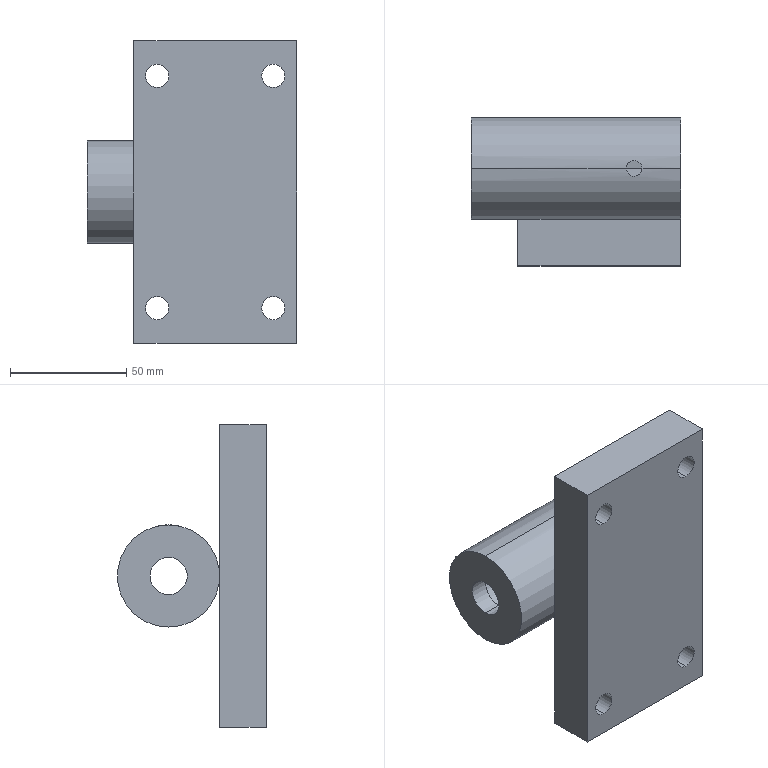Part | SolidWorks | features MirrorStock 1 | 2 solids | 25 faces | box 90 x 64 x 130 mm | volume 252738 mm3 | cylinder 16 | plane 9 | commonest cylinder face diameters 10 x8 6.8 x2 16 x2 30 x2 44 x2
STEP:
#1=CARTESIAN_POINT('',(-25.,20.,45.));
#2=VERTEX_POINT('',#1);
#3=CARTESIAN_POINT('',(-25.,20.,55.));
#4=VERTEX_POINT('',#3);
#5=CARTESIAN_POINT('',(-25.,20.,50.));
#6=DIRECTION('',(0.,-1.,0.));
#7=DIRECTION('',(0.,0.,-1.));
#8=AXIS2_PLACEMENT_3D('',#5,#6,#7);
#9=CIRCLE('',#8,5.);
#10=EDGE_CURVE('',#2,#4,#9,.T.);
#11=ORIENTED_EDGE('',*,*,#10,.F.);
#12=CARTESIAN_POINT('',(-25.,0.,45.));
#13=VERTEX_POINT('',#12);
#14=CARTESIAN_POINT('',(-25.,20.,45.));
#15=DIRECTION('',(0.,-1.,0.));
#16=VECTOR('',#15,1000.);
#17=LINE('',#14,#16);
#18=EDGE_CURVE('',#2,#13,#17,.T.);
#19=ORIENTED_EDGE('',*,*,#18,.T.);
#20=CARTESIAN_POINT('',(-25.,0.,55.));
#21=VERTEX_POINT('',#20);
#22=CARTESIAN_POINT('',(-25.,0.,50.));
#23=DIRECTION('',(0.,-1.,0.));
#24=DIRECTION('',(0.,0.,-1.));
#25=AXIS2_PLACEMENT_3D('',#22,#23,#24);
#26=CIRCLE('',#25,5.);
#27=EDGE_CURVE('',#13,#21,#26,.T.);
#28=ORIENTED_EDGE('',*,*,#27,.T.);
#29=CARTESIAN_POINT('',(-25.,20.,55.));
#30=DIRECTION('',(0.,-1.,0.));
#31=VECTOR('',#30,1000.);
#32=LINE('',#29,#31);
#33=EDGE_CURVE('',#4,#21,#32,.T.);
#34=ORIENTED_EDGE('',*,*,#33,.F.);
#35=EDGE_LOOP('',(#11,#19,#28,#34));
#36=FACE_OUTER_BOUND('',#35,.T.);
#37=CARTESIAN_POINT('',(-25.,20.,50.));
#38=DIRECTION('',(0.,-1.,0.));
#39=DIRECTION('',(0.,0.,1.));
#40=AXIS2_PLACEMENT_3D('',#37,#38,#39);
#41=CYLINDRICAL_SURFACE('',#40,5.);
#42=ADVANCED_FACE('',(#36),#41,.F.);
#43=CARTESIAN_POINT('',(25.,20.,45.));
#44=VERTEX_POINT('',#43);
#45=CARTESIAN_POINT('',(25.,20.,55.));
#46=VERTEX_POINT('',#45);
#47=CARTESIAN_POINT('',(25.,20.,50.));
#48=DIRECTION('',(0.,-1.,0.));
#49=DIRECTION('',(0.,0.,-1.));
#50=AXIS2_PLACEMENT_3D('',#47,#48,#49);
#51=CIRCLE('',#50,5.);
#52=EDGE_CURVE('',#44,#46,#51,.T.);
#53=ORIENTED_EDGE('',*,*,#52,.F.);
#54=CARTESIAN_POINT('',(25.,0.,45.));
#55=VERTEX_POINT('',#54);
#56=CARTESIAN_POINT('',(25.,20.,45.));
#57=DIRECTION('',(0.,-1.,0.));
#58=VECTOR('',#57,1000.);
#59=LINE('',#56,#58);
#60=EDGE_CURVE('',#44,#55,#59,.T.);
#61=ORIENTED_EDGE('',*,*,#60,.T.);
#62=CARTESIAN_POINT('',(25.,0.,55.));
#63=VERTEX_POINT('',#62);
#64=CARTESIAN_POINT('',(25.,0.,50.));
#65=DIRECTION('',(0.,-1.,0.));
#66=DIRECTION('',(0.,0.,-1.));
#67=AXIS2_PLACEMENT_3D('',#64,#65,#66);
#68=CIRCLE('',#67,5.);
#69=EDGE_CURVE('',#55,#63,#68,.T.);
#70=ORIENTED_EDGE('',*,*,#69,.T.);
#71=CARTESIAN_POINT('',(25.,20.,55.));
#72=DIRECTION('',(0.,-1.,0.));
#73=VECTOR('',#72,1000.);
#74=LINE('',#71,#73);
#75=EDGE_CURVE('',#46,#63,#74,.T.);
#76=ORIENTED_EDGE('',*,*,#75,.F.);
#77=EDGE_LOOP('',(#53,#61,#70,#76));
#78=FACE_OUTER_BOUND('',#77,.T.);
#79=CARTESIAN_POINT('',(25.,20.,50.));
#80=DIRECTION('',(0.,-1.,0.));
#81=DIRECTION('',(0.,0.,1.));
#82=AXIS2_PLACEMENT_3D('',#79,#80,#81);
#83=CYLINDRICAL_SURFACE('',#82,5.);
#84=ADVANCED_FACE('',(#78),#83,.F.);
#85=CARTESIAN_POINT('',(25.,20.,-55.));
#86=VERTEX_POINT('',#85);
#87=CARTESIAN_POINT('',(25.,20.,-45.));
#88=VERTEX_POINT('',#87);
#89=CARTESIAN_POINT('',(25.,20.,-50.));
#90=DIRECTION('',(0.,-1.,0.));
#91=DIRECTION('',(0.,0.,-1.));
#92=AXIS2_PLACEMENT_3D('',#89,#90,#91);
#93=CIRCLE('',#92,5.);
#94=EDGE_CURVE('',#86,#88,#93,.T.);
#95=ORIENTED_EDGE('',*,*,#94,.F.);
#96=CARTESIAN_POINT('',(25.,0.,-55.));
#97=VERTEX_POINT('',#96);
#98=CARTESIAN_POINT('',(25.,20.,-55.));
#99=DIRECTION('',(0.,-1.,0.));
#100=VECTOR('',#99,1000.);
#101=LINE('',#98,#100);
#102=EDGE_CURVE('',#86,#97,#101,.T.);
#103=ORIENTED_EDGE('',*,*,#102,.T.);
#104=CARTESIAN_POINT('',(25.,0.,-45.));
#105=VERTEX_POINT('',#104);
#106=CARTESIAN_POINT('',(25.,0.,-50.));
#107=DIRECTION('',(0.,-1.,0.));
#108=DIRECTION('',(0.,0.,-1.));
#109=AXIS2_PLACEMENT_3D('',#106,#107,#108);
#110=CIRCLE('',#109,5.);
#111=EDGE_CURVE('',#97,#105,#110,.T.);
#112=ORIENTED_EDGE('',*,*,#111,.T.);
#113=CARTESIAN_POINT('',(25.,20.,-45.));
#114=DIRECTION('',(0.,-1.,0.));
#115=VECTOR('',#114,1000.);
#116=LINE('',#113,#115);
#117=EDGE_CURVE('',#88,#105,#116,.T.);
#118=ORIENTED_EDGE('',*,*,#117,.F.);
#119=EDGE_LOOP('',(#95,#103,#112,#118));
#120=FACE_OUTER_BOUND('',#119,.T.);
#121=CARTESIAN_POINT('',(25.,20.,-50.));
#122=DIRECTION('',(0.,-1.,0.));
#123=DIRECTION('',(0.,0.,1.));
#124=AXIS2_PLACEMENT_3D('',#121,#122,#123);
#125=CYLINDRICAL_SURFACE('',#124,5.);
#126=ADVANCED_FACE('',(#120),#125,.F.);
#127=CARTESIAN_POINT('',(-25.,20.,-55.));
#128=VERTEX_POINT('',#127);
#129=CARTESIAN_POINT('',(-25.,20.,-45.));
#130=VERTEX_POINT('',#129);
#131=CARTESIAN_POINT('',(-25.,20.,-50.));
#132=DIRECTION('',(0.,-1.,0.));
#133=DIRECTION('',(0.,0.,-1.));
#134=AXIS2_PLACEMENT_3D('',#131,#132,#133);
#135=CIRCLE('',#134,5.);
#136=EDGE_CURVE('',#128,#130,#135,.T.);
#137=ORIENTED_EDGE('',*,*,#136,.F.);
#138=CARTESIAN_POINT('',(-25.,0.,-55.));
#139=VERTEX_POINT('',#138);
#140=CARTESIAN_POINT('',(-25.,20.,-55.));
#141=DIRECTION('',(0.,-1.,0.));
#142=VECTOR('',#141,1000.);
#143=LINE('',#140,#142);
#144=EDGE_CURVE('',#128,#139,#143,.T.);
#145=ORIENTED_EDGE('',*,*,#144,.T.);
#146=CARTESIAN_POINT('',(-25.,0.,-45.));
#147=VERTEX_POINT('',#146);
#148=CARTESIAN_POINT('',(-25.,0.,-50.));
#149=DIRECTION('',(0.,-1.,0.));
#150=DIRECTION('',(0.,0.,-1.));
#151=AXIS2_PLACEMENT_3D('',#148,#149,#150);
#152=CIRCLE('',#151,5.);
#153=EDGE_CURVE('',#139,#147,#152,.T.);
#154=ORIENTED_EDGE('',*,*,#153,.T.);
#155=CARTESIAN_POINT('',(-25.,20.,-45.));
#156=DIRECTION('',(0.,-1.,0.));
#157=VECTOR('',#156,1000.);
#158=LINE('',#155,#157);
#159=EDGE_CURVE('',#130,#147,#158,.T.);
#160=ORIENTED_EDGE('',*,*,#159,.F.);
#161=EDGE_LOOP('',(#137,#145,#154,#160));
#162=FACE_OUTER_BOUND('',#161,.T.);
#163=CARTESIAN_POINT('',(-25.,20.,-50.));
#164=DIRECTION('',(0.,-1.,0.));
#165=DIRECTION('',(0.,0.,1.));
#166=AXIS2_PLACEMENT_3D('',#163,#164,#165);
#167=CYLINDRICAL_SURFACE('',#166,5.);
#168=ADVANCED_FACE('',(#162),#167,.F.);
#169=CARTESIAN_POINT('',(-35.,20.,65.));
#170=VERTEX_POINT('',#169);
#171=CARTESIAN_POINT('',(-35.,20.,-65.));
#172=VERTEX_POINT('',#171);
#173=CARTESIAN_POINT('',(-35.,20.,-65.));
#174=DIRECTION('',(0.,0.,-1.));
#175=VECTOR('',#174,1000.);
#176=LINE('',#173,#175);
#177=EDGE_CURVE('',#170,#172,#176,.T.);
#178=ORIENTED_EDGE('',*,*,#177,.F.);
#179=CARTESIAN_POINT('',(35.,20.,65.));
#180=VERTEX_POINT('',#179);
#181=CARTESIAN_POINT('',(-35.,20.,65.));
#182=DIRECTION('',(-1.,0.,0.));
#183=VECTOR('',#182,1000.);
#184=LINE('',#181,#183);
#185=EDGE_CURVE('',#180,#170,#184,.T.);
#186=ORIENTED_EDGE('',*,*,#185,.F.);
#187=CARTESIAN_POINT('',(35.,20.,-65.));
#188=VERTEX_POINT('',#187);
#189=CARTESIAN_POINT('',(35.,20.,-65.));
#190=DIRECTION('',(0.,0.,1.));
#191=VECTOR('',#190,1000.);
#192=LINE('',#189,#191);
#193=EDGE_CURVE('',#188,#180,#192,.T.);
#194=ORIENTED_EDGE('',*,*,#193,.F.);
#195=CARTESIAN_POINT('',(-35.,20.,-65.));
#196=DIRECTION('',(1.,0.,0.));
#197=VECTOR('',#196,1000.);
#198=LINE('',#195,#197);
#199=EDGE_CURVE('',#172,#188,#198,.T.);
#200=ORIENTED_EDGE('',*,*,#199,.F.);
#201=EDGE_LOOP('',(#178,#186,#194,#200));
#202=FACE_OUTER_BOUND('',#201,.T.);
#203=CARTESIAN_POINT('',(25.,20.,50.));
#204=DIRECTION('',(0.,-1.,0.));
#205=DIRECTION('',(0.,0.,-1.));
#206=AXIS2_PLACEMENT_3D('',#203,#204,#205);
#207=CIRCLE('',#206,5.);
#208=EDGE_CURVE('',#46,#44,#207,.T.);
#209=ORIENTED_EDGE('',*,*,#208,.T.);
#210=ORIENTED_EDGE('',*,*,#52,.T.);
#211=EDGE_LOOP('',(#209,#210));
#212=FACE_BOUND('',#211,.T.);
#213=CARTESIAN_POINT('',(-25.,20.,50.));
#214=DIRECTION('',(0.,-1.,0.));
#215=DIRECTION('',(0.,0.,-1.));
#216=AXIS2_PLACEMENT_3D('',#213,#214,#215);
#217=CIRCLE('',#216,5.);
#218=EDGE_CURVE('',#4,#2,#217,.T.);
#219=ORIENTED_EDGE('',*,*,#218,.T.);
#220=ORIENTED_EDGE('',*,*,#10,.T.);
#221=EDGE_LOOP('',(#219,#220));
#222=FACE_BOUND('',#221,.T.);
#223=CARTESIAN_POINT('',(25.,20.,-50.));
#224=DIRECTION('',(0.,-1.,0.));
#225=DIRECTION('',(0.,0.,-1.));
#226=AXIS2_PLACEMENT_3D('',#223,#224,#225);
#227=CIRCLE('',#226,5.);
#228=EDGE_CURVE('',#88,#86,#227,.T.);
#229=ORIENTED_EDGE('',*,*,#228,.T.);
#230=ORIENTED_EDGE('',*,*,#94,.T.);
#231=EDGE_LOOP('',(#229,#230));
#232=FACE_BOUND('',#231,.T.);
#233=CARTESIAN_POINT('',(-25.,20.,-50.));
#234=DIRECTION('',(0.,-1.,0.));
#235=DIRECTION('',(0.,0.,-1.));
#236=AXIS2_PLACEMENT_3D('',#233,#234,#235);
#237=CIRCLE('',#236,5.);
#238=EDGE_CURVE('',#130,#128,#237,.T.);
#239=ORIENTED_EDGE('',*,*,#238,.T.);
#240=ORIENTED_EDGE('',*,*,#136,.T.);
#241=EDGE_LOOP('',(#239,#240));
#242=FACE_BOUND('',#241,.T.);
#243=CARTESIAN_POINT('',(0.,20.,0.));
#244=DIRECTION('',(0.,-1.,0.));
#245=DIRECTION('',(0.,0.,1.));
#246=AXIS2_PLACEMENT_3D('',#243,#244,#245);
#247=PLANE('',#246);
#248=ADVANCED_FACE('',(#202,#212,#222,#232,#242),#247,.F.);
#249=CARTESIAN_POINT('',(25.,0.,50.));
#250=DIRECTION('',(0.,-1.,0.));
#251=DIRECTION('',(0.,0.,-1.));
#252=AXIS2_PLACEMENT_3D('',#249,#250,#251);
#253=CIRCLE('',#252,5.);
#254=EDGE_CURVE('',#63,#55,#253,.T.);
#255=ORIENTED_EDGE('',*,*,#254,.F.);
#256=ORIENTED_EDGE('',*,*,#69,.F.);
#257=EDGE_LOOP('',(#255,#256));
#258=FACE_BOUND('',#257,.T.);
#259=CARTESIAN_POINT('',(-25.,0.,-50.));
#260=DIRECTION('',(0.,-1.,0.));
#261=DIRECTION('',(0.,0.,-1.));
#262=AXIS2_PLACEMENT_3D('',#259,#260,#261);
#263=CIRCLE('',#262,5.);
#264=EDGE_CURVE('',#147,#139,#263,.T.);
#265=ORIENTED_EDGE('',*,*,#264,.F.);
#266=ORIENTED_EDGE('',*,*,#153,.F.);
#267=EDGE_LOOP('',(#265,#266));
#268=FACE_BOUND('',#267,.T.);
#269=CARTESIAN_POINT('',(35.,0.,-65.));
#270=VERTEX_POINT('',#269);
#271=CARTESIAN_POINT('',(35.,0.,65.));
#272=VERTEX_POINT('',#271);
#273=CARTESIAN_POINT('',(35.,0.,-65.));
#274=DIRECTION('',(0.,0.,1.));
#275=VECTOR('',#274,1000.);
#276=LINE('',#273,#275);
#277=EDGE_CURVE('',#270,#272,#276,.T.);
#278=ORIENTED_EDGE('',*,*,#277,.T.);
#279=CARTESIAN_POINT('',(-35.,0.,65.));
#280=VERTEX_POINT('',#279);
#281=CARTESIAN_POINT('',(-35.,0.,65.));
#282=DIRECTION('',(-1.,0.,0.));
#283=VECTOR('',#282,1000.);
#284=LINE('',#281,#283);
#285=EDGE_CURVE('',#272,#280,#284,.T.);
#286=ORIENTED_EDGE('',*,*,#285,.T.);
#287=CARTESIAN_POINT('',(-35.,0.,-65.));
#288=VERTEX_POINT('',#287);
#289=CARTESIAN_POINT('',(-35.,0.,-65.));
#290=DIRECTION('',(0.,0.,-1.));
#291=VECTOR('',#290,1000.);
#292=LINE('',#289,#291);
#293=EDGE_CURVE('',#280,#288,#292,.T.);
#294=ORIENTED_EDGE('',*,*,#293,.T.);
#295=CARTESIAN_POINT('',(-35.,0.,-65.));
#296=DIRECTION('',(1.,0.,0.));
#297=VECTOR('',#296,1000.);
#298=LINE('',#295,#297);
#299=EDGE_CURVE('',#288,#270,#298,.T.);
#300=ORIENTED_EDGE('',*,*,#299,.T.);
#301=EDGE_LOOP('',(#278,#286,#294,#300));
#302=FACE_OUTER_BOUND('',#301,.T.);
#303=CARTESIAN_POINT('',(25.,0.,-50.));
#304=DIRECTION('',(0.,-1.,0.));
#305=DIRECTION('',(0.,0.,-1.));
#306=AXIS2_PLACEMENT_3D('',#303,#304,#305);
#307=CIRCLE('',#306,5.);
#308=EDGE_CURVE('',#105,#97,#307,.T.);
#309=ORIENTED_EDGE('',*,*,#308,.F.);
#310=ORIENTED_EDGE('',*,*,#111,.F.);
#311=EDGE_LOOP('',(#309,#310));
#312=FACE_BOUND('',#311,.T.);
#313=CARTESIAN_POINT('',(-25.,0.,50.));
#314=DIRECTION('',(0.,-1.,0.));
#315=DIRECTION('',(0.,0.,-1.));
#316=AXIS2_PLACEMENT_3D('',#313,#314,#315);
#317=CIRCLE('',#316,5.);
#318=EDGE_CURVE('',#21,#13,#317,.T.);
#319=ORIENTED_EDGE('',*,*,#318,.F.);
#320=ORIENTED_EDGE('',*,*,#27,.F.);
#321=EDGE_LOOP('',(#319,#320));
#322=FACE_BOUND('',#321,.T.);
#323=CARTESIAN_POINT('',(0.,0.,0.));
#324=DIRECTION('',(0.,-1.,0.));
#325=DIRECTION('',(0.,0.,1.));
#326=AXIS2_PLACEMENT_3D('',#323,#324,#325);
#327=PLANE('',#326);
#328=ADVANCED_FACE('',(#258,#268,#302,#312,#322),#327,.T.);
#329=ORIENTED_EDGE('',*,*,#277,.F.);
#330=CARTESIAN_POINT('',(35.,20.,-65.));
#331=DIRECTION('',(0.,-1.,0.));
#332=VECTOR('',#331,1000.);
#333=LINE('',#330,#332);
#334=EDGE_CURVE('',#188,#270,#333,.T.);
#335=ORIENTED_EDGE('',*,*,#334,.F.);
#336=ORIENTED_EDGE('',*,*,#193,.T.);
#337=CARTESIAN_POINT('',(35.,20.,65.));
#338=DIRECTION('',(0.,-1.,0.));
#339=VECTOR('',#338,1000.);
#340=LINE('',#337,#339);
#341=EDGE_CURVE('',#180,#272,#340,.T.);
#342=ORIENTED_EDGE('',*,*,#341,.T.);
#343=EDGE_LOOP('',(#329,#335,#336,#342));
#344=FACE_OUTER_BOUND('',#343,.T.);
#345=CARTESIAN_POINT('',(35.,20.,-65.));
#346=DIRECTION('',(-1.,0.,0.));
#347=DIRECTION('',(0.,0.,-1.));
#348=AXIS2_PLACEMENT_3D('',#345,#346,#347);
#349=PLANE('',#348);
#350=ADVANCED_FACE('',(#344),#349,.F.);
#351=ORIENTED_EDGE('',*,*,#285,.F.);
#352=ORIENTED_EDGE('',*,*,#341,.F.);
#353=ORIENTED_EDGE('',*,*,#185,.T.);
#354=CARTESIAN_POINT('',(-35.,20.,65.));
#355=DIRECTION('',(0.,-1.,0.));
#356=VECTOR('',#355,1000.);
#357=LINE('',#354,#356);
#358=EDGE_CURVE('',#170,#280,#357,.T.);
#359=ORIENTED_EDGE('',*,*,#358,.T.);
#360=EDGE_LOOP('',(#351,#352,#353,#359));
#361=FACE_OUTER_BOUND('',#360,.T.);
#362=CARTESIAN_POINT('',(-35.,20.,65.));
#363=DIRECTION('',(0.,0.,-1.));
#364=DIRECTION('',(1.,0.,0.));
#365=AXIS2_PLACEMENT_3D('',#362,#363,#364);
#366=PLANE('',#365);
#367=ADVANCED_FACE('',(#361),#366,.F.);
#368=ORIENTED_EDGE('',*,*,#293,.F.);
#369=ORIENTED_EDGE('',*,*,#358,.F.);
#370=ORIENTED_EDGE('',*,*,#177,.T.);
#371=CARTESIAN_POINT('',(-35.,20.,-65.));
#372=DIRECTION('',(0.,-1.,0.));
#373=VECTOR('',#372,1000.);
#374=LINE('',#371,#373);
#375=EDGE_CURVE('',#172,#288,#374,.T.);
#376=ORIENTED_EDGE('',*,*,#375,.T.);
#377=EDGE_LOOP('',(#368,#369,#370,#376));
#378=FACE_OUTER_BOUND('',#377,.T.);
#379=CARTESIAN_POINT('',(-35.,20.,-65.));
#380=DIRECTION('',(1.,0.,0.));
#381=DIRECTION('',(0.,0.,1.));
#382=AXIS2_PLACEMENT_3D('',#379,#380,#381);
#383=PLANE('',#382);
#384=ADVANCED_FACE('',(#378),#383,.F.);
#385=ORIENTED_EDGE('',*,*,#299,.F.);
#386=ORIENTED_EDGE('',*,*,#375,.F.);
#387=ORIENTED_EDGE('',*,*,#199,.T.);
#388=ORIENTED_EDGE('',*,*,#334,.T.);
#389=EDGE_LOOP('',(#385,#386,#387,#388));
#390=FACE_OUTER_BOUND('',#389,.T.);
#391=CARTESIAN_POINT('',(-35.,20.,-65.));
#392=DIRECTION('',(0.,0.,1.));
#393=DIRECTION('',(-1.,0.,0.));
#394=AXIS2_PLACEMENT_3D('',#391,#392,#393);
#395=PLANE('',#394);
#396=ADVANCED_FACE('',(#390),#395,.F.);
#397=ORIENTED_EDGE('',*,*,#144,.F.);
#398=ORIENTED_EDGE('',*,*,#238,.F.);
#399=ORIENTED_EDGE('',*,*,#159,.T.);
#400=ORIENTED_EDGE('',*,*,#264,.T.);
#401=EDGE_LOOP('',(#397,#398,#399,#400));
#402=FACE_OUTER_BOUND('',#401,.T.);
#403=CARTESIAN_POINT('',(-25.,20.,-50.));
#404=DIRECTION('',(0.,-1.,0.));
#405=DIRECTION('',(0.,0.,1.));
#406=AXIS2_PLACEMENT_3D('',#403,#404,#405);
#407=CYLINDRICAL_SURFACE('',#406,5.);
#408=ADVANCED_FACE('',(#402),#407,.F.);
#409=ORIENTED_EDGE('',*,*,#102,.F.);
#410=ORIENTED_EDGE('',*,*,#228,.F.);
#411=ORIENTED_EDGE('',*,*,#117,.T.);
#412=ORIENTED_EDGE('',*,*,#308,.T.);
#413=EDGE_LOOP('',(#409,#410,#411,#412));
#414=FACE_OUTER_BOUND('',#413,.T.);
#415=CARTESIAN_POINT('',(25.,20.,-50.));
#416=DIRECTION('',(0.,-1.,0.));
#417=DIRECTION('',(0.,0.,1.));
#418=AXIS2_PLACEMENT_3D('',#415,#416,#417);
#419=CYLINDRICAL_SURFACE('',#418,5.);
#420=ADVANCED_FACE('',(#414),#419,.F.);
#421=ORIENTED_EDGE('',*,*,#60,.F.);
#422=ORIENTED_EDGE('',*,*,#208,.F.);
#423=ORIENTED_EDGE('',*,*,#75,.T.);
#424=ORIENTED_EDGE('',*,*,#254,.T.);
#425=EDGE_LOOP('',(#421,#422,#423,#424));
#426=FACE_OUTER_BOUND('',#425,.T.);
#427=CARTESIAN_POINT('',(25.,20.,50.));
#428=DIRECTION('',(0.,-1.,0.));
#429=DIRECTION('',(0.,0.,1.));
#430=AXIS2_PLACEMENT_3D('',#427,#428,#429);
#431=CYLINDRICAL_SURFACE('',#430,5.);
#432=ADVANCED_FACE('',(#426),#431,.F.);
#433=ORIENTED_EDGE('',*,*,#18,.F.);
#434=ORIENTED_EDGE('',*,*,#218,.F.);
#435=ORIENTED_EDGE('',*,*,#33,.T.);
#436=ORIENTED_EDGE('',*,*,#318,.T.);
#437=EDGE_LOOP('',(#433,#434,#435,#436));
#438=FACE_OUTER_BOUND('',#437,.T.);
#439=CARTESIAN_POINT('',(-25.,20.,50.));
#440=DIRECTION('',(0.,-1.,0.));
#441=DIRECTION('',(0.,0.,1.));
#442=AXIS2_PLACEMENT_3D('',#439,#440,#441);
#443=CYLINDRICAL_SURFACE('',#442,5.);
#444=ADVANCED_FACE('',(#438),#443,.F.);
#445=CLOSED_SHELL('',(#42,#84,#126,#168,#248,#328,#350,#367,#384,#396,#408,#420,#432,#444));
#446=MANIFOLD_SOLID_BREP('',#445);
#447=CARTESIAN_POINT('',(18.4,42.,22.));
#448=VERTEX_POINT('',#447);
#449=CARTESIAN_POINT('',(11.6,42.,22.));
#450=VERTEX_POINT('',#449);
#451=CARTESIAN_POINT('',(18.4,42.,22.));
#452=CARTESIAN_POINT('',(18.4,42.225,22.));
#453=CARTESIAN_POINT('',(18.378,42.446,21.997));
#454=CARTESIAN_POINT('',(18.291,42.881,21.983));
#455=CARTESIAN_POINT('',(18.226,43.097,21.974));
#456=CARTESIAN_POINT('',(18.055,43.509,21.949));
#457=CARTESIAN_POINT('',(17.95,43.704,21.935));
#458=CARTESIAN_POINT('',(17.704,44.074,21.903));
#459=CARTESIAN_POINT('',(17.56,44.248,21.885));
#460=CARTESIAN_POINT('',(17.247,44.561,21.851));
#461=CARTESIAN_POINT('',(17.076,44.702,21.834));
#462=CARTESIAN_POINT('',(16.704,44.95,21.802));
#463=CARTESIAN_POINT('',(16.507,45.056,21.787));
#464=CARTESIAN_POINT('',(16.098,45.225,21.762));
#465=CARTESIAN_POINT('',(15.883,45.291,21.753));
#466=CARTESIAN_POINT('',(15.444,45.378,21.739));
#467=CARTESIAN_POINT('',(15.223,45.4,21.736));
#468=CARTESIAN_POINT('',(14.779,45.4,21.736));
#469=CARTESIAN_POINT('',(14.553,45.378,21.739));
#470=CARTESIAN_POINT('',(14.117,45.291,21.753));
#471=CARTESIAN_POINT('',(13.905,45.227,21.762));
#472=CARTESIAN_POINT('',(13.493,45.056,21.787));
#473=CARTESIAN_POINT('',(13.294,44.95,21.802));
#474=CARTESIAN_POINT('',(12.926,44.704,21.834));
#475=CARTESIAN_POINT('',(12.754,44.563,21.851));
#476=CARTESIAN_POINT('',(12.438,44.246,21.886));
#477=CARTESIAN_POINT('',(12.297,44.074,21.903));
#478=CARTESIAN_POINT('',(12.051,43.707,21.934));
#479=CARTESIAN_POINT('',(11.944,43.508,21.949));
#480=CARTESIAN_POINT('',(11.774,43.096,21.974));
#481=CARTESIAN_POINT('',(11.709,42.884,21.983));
#482=CARTESIAN_POINT('',(11.622,42.448,21.997));
#483=CARTESIAN_POINT('',(11.6,42.222,22.));
#484=CARTESIAN_POINT('',(11.6,42.,22.));
#485=B_SPLINE_CURVE_WITH_KNOTS('',3,(#451,#452,#453,#454,#455,#456,#457,#458,#459,#460,#461,#462,#463,#464,#465,#466,#467,#468,#469,#470,#471,#472,#473,#474,#475,#476,#477,#478,#479,#480,#481,#482,#483,#484),.UNSPECIFIED.,.F.,.F.,(4,2,2,2,2,2,2,2,2,2,2,2,2,2,2,2,4),(0.,0.0006654,0.001331,0.001996,0.002661,0.003327,0.003992,0.004658,0.005323,0.005988,0.006654,0.007319,0.007984,0.00865,0.009315,0.009981,0.01065),.UNSPECIFIED.);
#486=EDGE_CURVE('',#448,#450,#485,.T.);
#487=ORIENTED_EDGE('',*,*,#486,.T.);
#488=CARTESIAN_POINT('',(11.6,42.,15.));
#489=VERTEX_POINT('',#488);
#490=CARTESIAN_POINT('',(11.6,42.,0.));
#491=DIRECTION('',(0.,0.,-1.));
#492=VECTOR('',#491,1000.);
#493=LINE('',#490,#492);
#494=EDGE_CURVE('',#450,#489,#493,.T.);
#495=ORIENTED_EDGE('',*,*,#494,.T.);
#496=CARTESIAN_POINT('',(18.4,42.,15.));
#497=VERTEX_POINT('',#496);
#498=CARTESIAN_POINT('',(11.6,42.,15.));
#499=CARTESIAN_POINT('',(11.6,42.222,15.));
#500=CARTESIAN_POINT('',(11.622,42.444,14.995));
#501=CARTESIAN_POINT('',(11.709,42.885,14.976));
#502=CARTESIAN_POINT('',(11.775,43.098,14.961));
#503=CARTESIAN_POINT('',(11.944,43.507,14.925));
#504=CARTESIAN_POINT('',(12.051,43.706,14.904));
#505=CARTESIAN_POINT('',(12.298,44.076,14.857));
#506=CARTESIAN_POINT('',(12.438,44.246,14.832));
#507=CARTESIAN_POINT('',(12.751,44.56,14.781));
#508=CARTESIAN_POINT('',(12.926,44.703,14.755));
#509=CARTESIAN_POINT('',(13.293,44.949,14.708));
#510=CARTESIAN_POINT('',(13.488,45.054,14.686));
#511=CARTESIAN_POINT('',(14.108,45.311,14.631));
#512=CARTESIAN_POINT('',(14.55,45.4,14.61));
#513=CARTESIAN_POINT('',(15.223,45.4,14.61));
#514=CARTESIAN_POINT('',(15.444,45.378,14.615));
#515=CARTESIAN_POINT('',(15.88,45.292,14.634));
#516=CARTESIAN_POINT('',(16.097,45.226,14.649));
#517=CARTESIAN_POINT('',(16.508,45.056,14.686));
#518=CARTESIAN_POINT('',(16.703,44.951,14.707));
#519=CARTESIAN_POINT('',(17.073,44.704,14.755));
#520=CARTESIAN_POINT('',(17.246,44.562,14.78));
#521=CARTESIAN_POINT('',(17.559,44.25,14.831));
#522=CARTESIAN_POINT('',(17.7,44.078,14.857));
#523=CARTESIAN_POINT('',(17.949,43.706,14.904));
#524=CARTESIAN_POINT('',(18.054,43.511,14.925));
#525=CARTESIAN_POINT('',(18.224,43.102,14.961));
#526=CARTESIAN_POINT('',(18.29,42.886,14.975));
#527=CARTESIAN_POINT('',(18.378,42.448,14.995));
#528=CARTESIAN_POINT('',(18.4,42.225,15.));
#529=CARTESIAN_POINT('',(18.4,42.,15.));
#530=B_SPLINE_CURVE_WITH_KNOTS('',3,(#498,#499,#500,#501,#502,#503,#504,#505,#506,#507,#508,#509,#510,#511,#512,#513,#514,#515,#516,#517,#518,#519,#520,#521,#522,#523,#524,#525,#526,#527,#528,#529),.UNSPECIFIED.,.F.,.F.,(4,2,2,2,2,2,2,2,2,2,2,2,2,2,2,4),(0.01066,0.01133,0.012,0.01266,0.01333,0.014,0.01466,0.016,0.01666,0.01733,0.01799,0.01866,0.01933,0.01999,0.02066,0.02133),.UNSPECIFIED.);
#531=EDGE_CURVE('',#489,#497,#530,.T.);
#532=ORIENTED_EDGE('',*,*,#531,.T.);
#533=CARTESIAN_POINT('',(18.4,42.,0.));
#534=DIRECTION('',(0.,0.,-1.));
#535=VECTOR('',#534,1000.);
#536=LINE('',#533,#535);
#537=EDGE_CURVE('',#448,#497,#536,.T.);
#538=ORIENTED_EDGE('',*,*,#537,.F.);
#539=EDGE_LOOP('',(#487,#495,#532,#538));
#540=FACE_OUTER_BOUND('',#539,.T.);
#541=CARTESIAN_POINT('',(15.,42.,0.));
#542=DIRECTION('',(0.,0.,-1.));
#543=DIRECTION('',(1.,0.,0.));
#544=AXIS2_PLACEMENT_3D('',#541,#542,#543);
#545=CYLINDRICAL_SURFACE('',#544,3.4);
#546=ADVANCED_FACE('',(#540),#545,.F.);
#547=CARTESIAN_POINT('',(-47.,42.,-8.));
#548=VERTEX_POINT('',#547);
#549=CARTESIAN_POINT('',(-47.,42.,8.));
#550=VERTEX_POINT('',#549);
#551=CARTESIAN_POINT('',(-47.,42.,0.));
#552=DIRECTION('',(1.,0.,0.));
#553=DIRECTION('',(0.,0.,-1.));
#554=AXIS2_PLACEMENT_3D('',#551,#552,#553);
#555=CIRCLE('',#554,8.);
#556=EDGE_CURVE('',#548,#550,#555,.T.);
#557=ORIENTED_EDGE('',*,*,#556,.T.);
#558=CARTESIAN_POINT('',(-55.,42.,8.));
#559=VERTEX_POINT('',#558);
#560=CARTESIAN_POINT('',(-55.,42.,8.));
#561=DIRECTION('',(-1.,0.,0.));
#562=VECTOR('',#561,1000.);
#563=LINE('',#560,#562);
#564=EDGE_CURVE('',#550,#559,#563,.T.);
#565=ORIENTED_EDGE('',*,*,#564,.T.);
#566=CARTESIAN_POINT('',(-55.,42.,-8.));
#567=VERTEX_POINT('',#566);
#568=CARTESIAN_POINT('',(-55.,42.,0.));
#569=DIRECTION('',(1.,0.,0.));
#570=DIRECTION('',(0.,0.,-1.));
#571=AXIS2_PLACEMENT_3D('',#568,#569,#570);
#572=CIRCLE('',#571,8.);
#573=EDGE_CURVE('',#567,#559,#572,.T.);
#574=ORIENTED_EDGE('',*,*,#573,.F.);
#575=CARTESIAN_POINT('',(-55.,42.,-8.));
#576=DIRECTION('',(-1.,0.,0.));
#577=VECTOR('',#576,1000.);
#578=LINE('',#575,#577);
#579=EDGE_CURVE('',#548,#567,#578,.T.);
#580=ORIENTED_EDGE('',*,*,#579,.F.);
#581=EDGE_LOOP('',(#557,#565,#574,#580));
#582=FACE_OUTER_BOUND('',#581,.T.);
#583=CARTESIAN_POINT('',(-55.,42.,0.));
#584=DIRECTION('',(-1.,0.,0.));
#585=DIRECTION('',(0.,0.,-1.));
#586=AXIS2_PLACEMENT_3D('',#583,#584,#585);
#587=CYLINDRICAL_SURFACE('',#586,8.);
#588=ADVANCED_FACE('',(#582),#587,.F.);
#589=CARTESIAN_POINT('',(35.,42.,22.));
#590=VERTEX_POINT('',#589);
#591=CARTESIAN_POINT('',(35.,42.,-22.));
#592=VERTEX_POINT('',#591);
#593=CARTESIAN_POINT('',(35.,42.,0.));
#594=DIRECTION('',(1.,0.,0.));
#595=DIRECTION('',(0.,0.,-1.));
#596=AXIS2_PLACEMENT_3D('',#593,#594,#595);
#597=CIRCLE('',#596,22.);
#598=EDGE_CURVE('',#590,#592,#597,.T.);
#599=ORIENTED_EDGE('',*,*,#598,.F.);
#600=CARTESIAN_POINT('',(-55.,42.,22.));
#601=DIRECTION('',(-1.,0.,0.));
#602=VECTOR('',#601,1000.);
#603=LINE('',#600,#602);
#604=EDGE_CURVE('',#590,#448,#603,.T.);
#605=ORIENTED_EDGE('',*,*,#604,.T.);
#606=CARTESIAN_POINT('',(11.6,42.,22.));
#607=CARTESIAN_POINT('',(11.6,41.778,22.));
#608=CARTESIAN_POINT('',(11.622,41.557,21.997));
#609=CARTESIAN_POINT('',(11.709,41.118,21.983));
#610=CARTESIAN_POINT('',(11.774,40.903,21.974));
#611=CARTESIAN_POINT('',(11.944,40.494,21.949));
#612=CARTESIAN_POINT('',(12.049,40.296,21.935));
#613=CARTESIAN_POINT('',(12.297,39.925,21.903));
#614=CARTESIAN_POINT('',(12.438,39.754,21.886));
#615=CARTESIAN_POINT('',(12.751,39.441,21.851));
#616=CARTESIAN_POINT('',(12.926,39.297,21.834));
#617=CARTESIAN_POINT('',(13.294,39.051,21.802));
#618=CARTESIAN_POINT('',(13.489,38.946,21.787));
#619=CARTESIAN_POINT('',(13.901,38.775,21.762));
#620=CARTESIAN_POINT('',(14.117,38.709,21.753));
#621=CARTESIAN_POINT('',(14.551,38.622,21.739));
#622=CARTESIAN_POINT('',(14.773,38.6,21.736));
#623=CARTESIAN_POINT('',(15.223,38.6,21.736));
#624=CARTESIAN_POINT('',(15.444,38.622,21.739));
#625=CARTESIAN_POINT('',(15.879,38.708,21.752));
#626=CARTESIAN_POINT('',(16.095,38.773,21.762));
#627=CARTESIAN_POINT('',(16.506,38.944,21.787));
#628=CARTESIAN_POINT('',(16.702,39.048,21.801));
#629=CARTESIAN_POINT('',(17.071,39.295,21.833));
#630=CARTESIAN_POINT('',(17.246,39.438,21.851));
#631=CARTESIAN_POINT('',(17.559,39.751,21.885));
#632=CARTESIAN_POINT('',(17.7,39.921,21.902));
#633=CARTESIAN_POINT('',(17.949,40.293,21.934));
#634=CARTESIAN_POINT('',(18.054,40.49,21.949));
#635=CARTESIAN_POINT('',(18.224,40.899,21.973));
#636=CARTESIAN_POINT('',(18.29,41.114,21.983));
#637=CARTESIAN_POINT('',(18.378,41.553,21.997));
#638=CARTESIAN_POINT('',(18.4,41.775,22.));
#639=CARTESIAN_POINT('',(18.4,42.,22.));
#640=B_SPLINE_CURVE_WITH_KNOTS('',3,(#606,#607,#608,#609,#610,#611,#612,#613,#614,#615,#616,#617,#618,#619,#620,#621,#622,#623,#624,#625,#626,#627,#628,#629,#630,#631,#632,#633,#634,#635,#636,#637,#638,#639),.UNSPECIFIED.,.F.,.F.,(4,2,2,2,2,2,2,2,2,2,2,2,2,2,2,2,4),(0.01065,0.01131,0.01198,0.01264,0.01331,0.01397,0.01464,0.0153,0.01597,0.01663,0.0173,0.01796,0.01863,0.01929,0.01996,0.02062,0.02129),.UNSPECIFIED.);
#641=EDGE_CURVE('',#450,#448,#640,.T.);
#642=ORIENTED_EDGE('',*,*,#641,.F.);
#643=CARTESIAN_POINT('',(-55.,42.,22.));
#644=VERTEX_POINT('',#643);
#645=CARTESIAN_POINT('',(-55.,42.,22.));
#646=DIRECTION('',(-1.,0.,0.));
#647=VECTOR('',#646,1000.);
#648=LINE('',#645,#647);
#649=EDGE_CURVE('',#450,#644,#648,.T.);
#650=ORIENTED_EDGE('',*,*,#649,.T.);
#651=CARTESIAN_POINT('',(-55.,42.,-22.));
#652=VERTEX_POINT('',#651);
#653=CARTESIAN_POINT('',(-55.,42.,0.));
#654=DIRECTION('',(1.,0.,0.));
#655=DIRECTION('',(0.,0.,-1.));
#656=AXIS2_PLACEMENT_3D('',#653,#654,#655);
#657=CIRCLE('',#656,22.);
#658=EDGE_CURVE('',#644,#652,#657,.T.);
#659=ORIENTED_EDGE('',*,*,#658,.T.);
#660=CARTESIAN_POINT('',(-55.,42.,-22.));
#661=DIRECTION('',(-1.,0.,0.));
#662=VECTOR('',#661,1000.);
#663=LINE('',#660,#662);
#664=EDGE_CURVE('',#592,#652,#663,.T.);
#665=ORIENTED_EDGE('',*,*,#664,.F.);
#666=EDGE_LOOP('',(#599,#605,#642,#650,#659,#665));
#667=FACE_OUTER_BOUND('',#666,.T.);
#668=CARTESIAN_POINT('',(-55.,42.,0.));
#669=DIRECTION('',(-1.,0.,0.));
#670=DIRECTION('',(0.,0.,-1.));
#671=AXIS2_PLACEMENT_3D('',#668,#669,#670);
#672=CYLINDRICAL_SURFACE('',#671,22.);
#673=ADVANCED_FACE('',(#667),#672,.T.);
#674=CARTESIAN_POINT('',(35.,42.,-15.));
#675=VERTEX_POINT('',#674);
#676=CARTESIAN_POINT('',(35.,42.,15.));
#677=VERTEX_POINT('',#676);
#678=CARTESIAN_POINT('',(35.,42.,0.));
#679=DIRECTION('',(1.,0.,0.));
#680=DIRECTION('',(0.,0.,-1.));
#681=AXIS2_PLACEMENT_3D('',#678,#679,#680);
#682=CIRCLE('',#681,15.);
#683=EDGE_CURVE('',#675,#677,#682,.T.);
#684=ORIENTED_EDGE('',*,*,#683,.T.);
#685=CARTESIAN_POINT('',(-55.,42.,15.));
#686=DIRECTION('',(-1.,0.,0.));
#687=VECTOR('',#686,1000.);
#688=LINE('',#685,#687);
#689=EDGE_CURVE('',#677,#497,#688,.T.);
#690=ORIENTED_EDGE('',*,*,#689,.T.);
#691=ORIENTED_EDGE('',*,*,#531,.F.);
#692=CARTESIAN_POINT('',(-47.,42.,15.));
#693=VERTEX_POINT('',#692);
#694=CARTESIAN_POINT('',(-55.,42.,15.));
#695=DIRECTION('',(-1.,0.,0.));
#696=VECTOR('',#695,1000.);
#697=LINE('',#694,#696);
#698=EDGE_CURVE('',#489,#693,#697,.T.);
#699=ORIENTED_EDGE('',*,*,#698,.T.);
#700=CARTESIAN_POINT('',(-47.,42.,-15.));
#701=VERTEX_POINT('',#700);
#702=CARTESIAN_POINT('',(-47.,42.,0.));
#703=DIRECTION('',(1.,0.,0.));
#704=DIRECTION('',(0.,0.,-1.));
#705=AXIS2_PLACEMENT_3D('',#702,#703,#704);
#706=CIRCLE('',#705,15.);
#707=EDGE_CURVE('',#701,#693,#706,.T.);
#708=ORIENTED_EDGE('',*,*,#707,.F.);
#709=CARTESIAN_POINT('',(-55.,42.,-15.));
#710=DIRECTION('',(-1.,0.,0.));
#711=VECTOR('',#710,1000.);
#712=LINE('',#709,#711);
#713=EDGE_CURVE('',#675,#701,#712,.T.);
#714=ORIENTED_EDGE('',*,*,#713,.F.);
#715=EDGE_LOOP('',(#684,#690,#691,#699,#708,#714));
#716=FACE_OUTER_BOUND('',#715,.T.);
#717=CARTESIAN_POINT('',(-55.,42.,0.));
#718=DIRECTION('',(-1.,0.,0.));
#719=DIRECTION('',(0.,0.,-1.));
#720=AXIS2_PLACEMENT_3D('',#717,#718,#719);
#721=CYLINDRICAL_SURFACE('',#720,15.);
#722=ADVANCED_FACE('',(#716),#721,.F.);
#723=ORIENTED_EDGE('',*,*,#707,.T.);
#724=CARTESIAN_POINT('',(-47.,42.,0.));
#725=DIRECTION('',(1.,0.,0.));
#726=DIRECTION('',(0.,0.,-1.));
#727=AXIS2_PLACEMENT_3D('',#724,#725,#726);
#728=CIRCLE('',#727,15.);
#729=EDGE_CURVE('',#693,#701,#728,.T.);
#730=ORIENTED_EDGE('',*,*,#729,.T.);
#731=EDGE_LOOP('',(#723,#730));
#732=FACE_OUTER_BOUND('',#731,.T.);
#733=ORIENTED_EDGE('',*,*,#556,.F.);
#734=CARTESIAN_POINT('',(-47.,42.,0.));
#735=DIRECTION('',(1.,0.,0.));
#736=DIRECTION('',(0.,0.,-1.));
#737=AXIS2_PLACEMENT_3D('',#734,#735,#736);
#738=CIRCLE('',#737,8.);
#739=EDGE_CURVE('',#550,#548,#738,.T.);
#740=ORIENTED_EDGE('',*,*,#739,.F.);
#741=EDGE_LOOP('',(#733,#740));
#742=FACE_BOUND('',#741,.T.);
#743=CARTESIAN_POINT('',(-47.,57.,0.));
#744=DIRECTION('',(-1.,0.,0.));
#745=DIRECTION('',(0.,0.,-1.));
#746=AXIS2_PLACEMENT_3D('',#743,#744,#745);
#747=PLANE('',#746);
#748=ADVANCED_FACE('',(#732,#742),#747,.F.);
#749=ORIENTED_EDGE('',*,*,#689,.F.);
#750=CARTESIAN_POINT('',(35.,42.,0.));
#751=DIRECTION('',(1.,0.,0.));
#752=DIRECTION('',(0.,0.,-1.));
#753=AXIS2_PLACEMENT_3D('',#750,#751,#752);
#754=CIRCLE('',#753,15.);
#755=EDGE_CURVE('',#677,#675,#754,.T.);
#756=ORIENTED_EDGE('',*,*,#755,.T.);
#757=ORIENTED_EDGE('',*,*,#713,.T.);
#758=ORIENTED_EDGE('',*,*,#729,.F.);
#759=ORIENTED_EDGE('',*,*,#698,.F.);
#760=CARTESIAN_POINT('',(18.4,42.,15.));
#761=CARTESIAN_POINT('',(18.4,41.775,15.));
#762=CARTESIAN_POINT('',(18.378,41.553,14.995));
#763=CARTESIAN_POINT('',(18.291,41.117,14.976));
#764=CARTESIAN_POINT('',(18.225,40.901,14.961));
#765=CARTESIAN_POINT('',(18.054,40.49,14.925));
#766=CARTESIAN_POINT('',(17.95,40.295,14.904));
#767=CARTESIAN_POINT('',(17.703,39.926,14.857));
#768=CARTESIAN_POINT('',(17.56,39.751,14.831));
#769=CARTESIAN_POINT('',(17.247,39.439,14.781));
#770=CARTESIAN_POINT('',(17.076,39.298,14.755));
#771=CARTESIAN_POINT('',(16.705,39.05,14.708));
#772=CARTESIAN_POINT('',(16.508,38.945,14.686));
#773=CARTESIAN_POINT('',(16.099,38.775,14.649));
#774=CARTESIAN_POINT('',(15.884,38.709,14.635));
#775=CARTESIAN_POINT('',(15.445,38.622,14.615));
#776=CARTESIAN_POINT('',(15.224,38.6,14.61));
#777=CARTESIAN_POINT('',(14.779,38.6,14.61));
#778=CARTESIAN_POINT('',(14.553,38.622,14.615));
#779=CARTESIAN_POINT('',(14.116,38.709,14.635));
#780=CARTESIAN_POINT('',(13.904,38.774,14.649));
#781=CARTESIAN_POINT('',(13.491,38.945,14.686));
#782=CARTESIAN_POINT('',(13.293,39.051,14.708));
#783=CARTESIAN_POINT('',(12.926,39.297,14.755));
#784=CARTESIAN_POINT('',(12.753,39.438,14.781));
#785=CARTESIAN_POINT('',(12.438,39.754,14.832));
#786=CARTESIAN_POINT('',(12.298,39.925,14.857));
#787=CARTESIAN_POINT('',(12.052,40.293,14.904));
#788=CARTESIAN_POINT('',(11.945,40.492,14.925));
#789=CARTESIAN_POINT('',(11.774,40.902,14.961));
#790=CARTESIAN_POINT('',(11.71,41.114,14.975));
#791=CARTESIAN_POINT('',(11.622,41.552,14.995));
#792=CARTESIAN_POINT('',(11.6,41.778,15.));
#793=CARTESIAN_POINT('',(11.6,42.,15.));
#794=B_SPLINE_CURVE_WITH_KNOTS('',3,(#760,#761,#762,#763,#764,#765,#766,#767,#768,#769,#770,#771,#772,#773,#774,#775,#776,#777,#778,#779,#780,#781,#782,#783,#784,#785,#786,#787,#788,#789,#790,#791,#792,#793),.UNSPECIFIED.,.F.,.F.,(4,2,2,2,2,2,2,2,2,2,2,2,2,2,2,2,4),(0.,0.0006665,0.001333,0.002,0.002666,0.003333,0.003999,0.004666,0.005332,0.005999,0.006665,0.007332,0.007999,0.008665,0.009332,0.009998,0.01066),.UNSPECIFIED.);
#795=EDGE_CURVE('',#497,#489,#794,.T.);
#796=ORIENTED_EDGE('',*,*,#795,.F.);
#797=EDGE_LOOP('',(#749,#756,#757,#758,#759,#796));
#798=FACE_OUTER_BOUND('',#797,.T.);
#799=CARTESIAN_POINT('',(-55.,42.,0.));
#800=DIRECTION('',(-1.,0.,0.));
#801=DIRECTION('',(0.,0.,-1.));
#802=AXIS2_PLACEMENT_3D('',#799,#800,#801);
#803=CYLINDRICAL_SURFACE('',#802,15.);
#804=ADVANCED_FACE('',(#798),#803,.F.);
#805=CARTESIAN_POINT('',(35.,42.,0.));
#806=DIRECTION('',(1.,0.,0.));
#807=DIRECTION('',(0.,0.,-1.));
#808=AXIS2_PLACEMENT_3D('',#805,#806,#807);
#809=CIRCLE('',#808,22.);
#810=EDGE_CURVE('',#592,#590,#809,.T.);
#811=ORIENTED_EDGE('',*,*,#810,.T.);
#812=ORIENTED_EDGE('',*,*,#598,.T.);
#813=EDGE_LOOP('',(#811,#812));
#814=FACE_OUTER_BOUND('',#813,.T.);
#815=ORIENTED_EDGE('',*,*,#683,.F.);
#816=ORIENTED_EDGE('',*,*,#755,.F.);
#817=EDGE_LOOP('',(#815,#816));
#818=FACE_BOUND('',#817,.T.);
#819=CARTESIAN_POINT('',(35.,64.,0.));
#820=DIRECTION('',(-1.,0.,0.));
#821=DIRECTION('',(0.,0.,-1.));
#822=AXIS2_PLACEMENT_3D('',#819,#820,#821);
#823=PLANE('',#822);
#824=ADVANCED_FACE('',(#814,#818),#823,.F.);
#825=ORIENTED_EDGE('',*,*,#604,.F.);
#826=ORIENTED_EDGE('',*,*,#810,.F.);
#827=ORIENTED_EDGE('',*,*,#664,.T.);
#828=CARTESIAN_POINT('',(-55.,42.,0.));
#829=DIRECTION('',(1.,0.,0.));
#830=DIRECTION('',(0.,0.,-1.));
#831=AXIS2_PLACEMENT_3D('',#828,#829,#830);
#832=CIRCLE('',#831,22.);
#833=EDGE_CURVE('',#652,#644,#832,.T.);
#834=ORIENTED_EDGE('',*,*,#833,.T.);
#835=ORIENTED_EDGE('',*,*,#649,.F.);
#836=ORIENTED_EDGE('',*,*,#486,.F.);
#837=EDGE_LOOP('',(#825,#826,#827,#834,#835,#836));
#838=FACE_OUTER_BOUND('',#837,.T.);
#839=CARTESIAN_POINT('',(-55.,42.,0.));
#840=DIRECTION('',(-1.,0.,0.));
#841=DIRECTION('',(0.,0.,-1.));
#842=AXIS2_PLACEMENT_3D('',#839,#840,#841);
#843=CYLINDRICAL_SURFACE('',#842,22.);
#844=ADVANCED_FACE('',(#838),#843,.T.);
#845=ORIENTED_EDGE('',*,*,#573,.T.);
#846=CARTESIAN_POINT('',(-55.,42.,0.));
#847=DIRECTION('',(1.,0.,0.));
#848=DIRECTION('',(0.,0.,-1.));
#849=AXIS2_PLACEMENT_3D('',#846,#847,#848);
#850=CIRCLE('',#849,8.);
#851=EDGE_CURVE('',#559,#567,#850,.T.);
#852=ORIENTED_EDGE('',*,*,#851,.T.);
#853=EDGE_LOOP('',(#845,#852));
#854=FACE_BOUND('',#853,.T.);
#855=ORIENTED_EDGE('',*,*,#833,.F.);
#856=ORIENTED_EDGE('',*,*,#658,.F.);
#857=EDGE_LOOP('',(#855,#856));
#858=FACE_OUTER_BOUND('',#857,.T.);
#859=CARTESIAN_POINT('',(-55.,50.,0.));
#860=DIRECTION('',(1.,0.,0.));
#861=DIRECTION('',(0.,0.,1.));
#862=AXIS2_PLACEMENT_3D('',#859,#860,#861);
#863=PLANE('',#862);
#864=ADVANCED_FACE('',(#854,#858),#863,.F.);
#865=ORIENTED_EDGE('',*,*,#564,.F.);
#866=ORIENTED_EDGE('',*,*,#739,.T.);
#867=ORIENTED_EDGE('',*,*,#579,.T.);
#868=ORIENTED_EDGE('',*,*,#851,.F.);
#869=EDGE_LOOP('',(#865,#866,#867,#868));
#870=FACE_OUTER_BOUND('',#869,.T.);
#871=CARTESIAN_POINT('',(-55.,42.,0.));
#872=DIRECTION('',(-1.,0.,0.));
#873=DIRECTION('',(0.,0.,-1.));
#874=AXIS2_PLACEMENT_3D('',#871,#872,#873);
#875=CYLINDRICAL_SURFACE('',#874,8.);
#876=ADVANCED_FACE('',(#870),#875,.F.);
#877=ORIENTED_EDGE('',*,*,#494,.F.);
#878=ORIENTED_EDGE('',*,*,#641,.T.);
#879=ORIENTED_EDGE('',*,*,#537,.T.);
#880=ORIENTED_EDGE('',*,*,#795,.T.);
#881=EDGE_LOOP('',(#877,#878,#879,#880));
#882=FACE_OUTER_BOUND('',#881,.T.);
#883=CARTESIAN_POINT('',(15.,42.,0.));
#884=DIRECTION('',(0.,0.,-1.));
#885=DIRECTION('',(1.,0.,0.));
#886=AXIS2_PLACEMENT_3D('',#883,#884,#885);
#887=CYLINDRICAL_SURFACE('',#886,3.4);
#888=ADVANCED_FACE('',(#882),#887,.F.);
#889=CLOSED_SHELL('',(#546,#588,#673,#722,#748,#804,#824,#844,#864,#876,#888));
#890=MANIFOLD_SOLID_BREP('',#889);
#891=CARTESIAN_POINT('',(0.,0.,0.));
#892=DIRECTION('',(0.,0.,1.));
#893=DIRECTION('',(1.,0.,0.));
#894=AXIS2_PLACEMENT_3D('',#891,#892,#893);
#895=(LENGTH_UNIT()NAMED_UNIT(*)SI_UNIT(.MILLI.,.METRE.));
#896=UNCERTAINTY_MEASURE_WITH_UNIT(LENGTH_MEASURE(0.00001),#895,'','');
#897=(NAMED_UNIT(*)PLANE_ANGLE_UNIT()SI_UNIT($,.RADIAN.));
#898=(NAMED_UNIT(*)SI_UNIT($,.STERADIAN.)SOLID_ANGLE_UNIT());
#899=(GEOMETRIC_REPRESENTATION_CONTEXT(3)GLOBAL_UNCERTAINTY_ASSIGNED_CONTEXT((#896))GLOBAL_UNIT_ASSIGNED_CONTEXT((#895,#897,#898))REPRESENTATION_CONTEXT('',''));
#900=ADVANCED_BREP_SHAPE_REPRESENTATION('',(#446,#890,#894),#899);